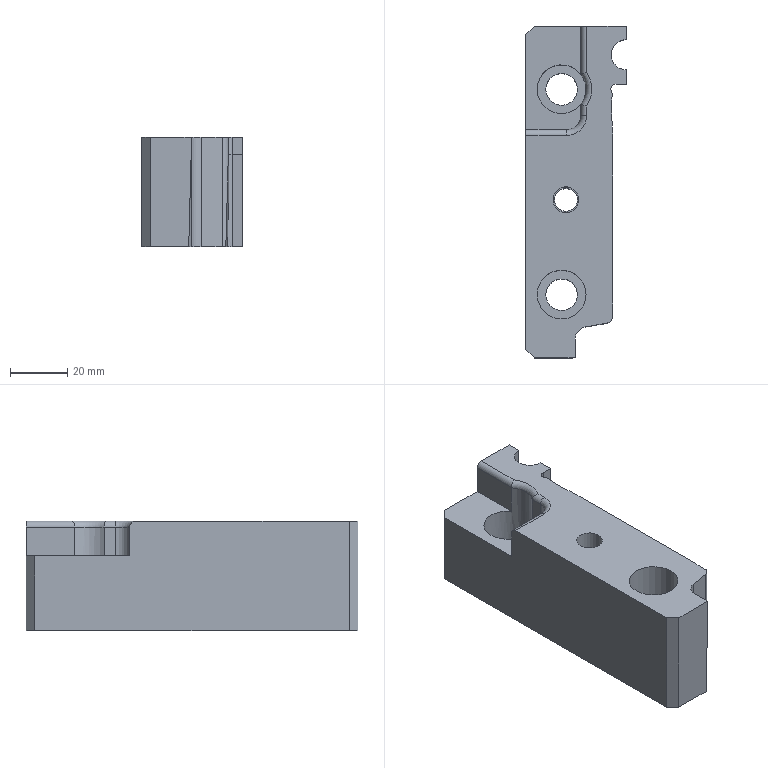Part | STEP file | 1_id122_x_t | 1 solid | 48 faces | box 35 x 115.5 x 38.1 mm | volume 107010 mm3 | plane 22 | cylinder 19 | cone 5 | torus 2 | commonest cylinder face diameters 4 x3 5.4 x2 11 x2 17 x2 2204 x2 2.4 x1